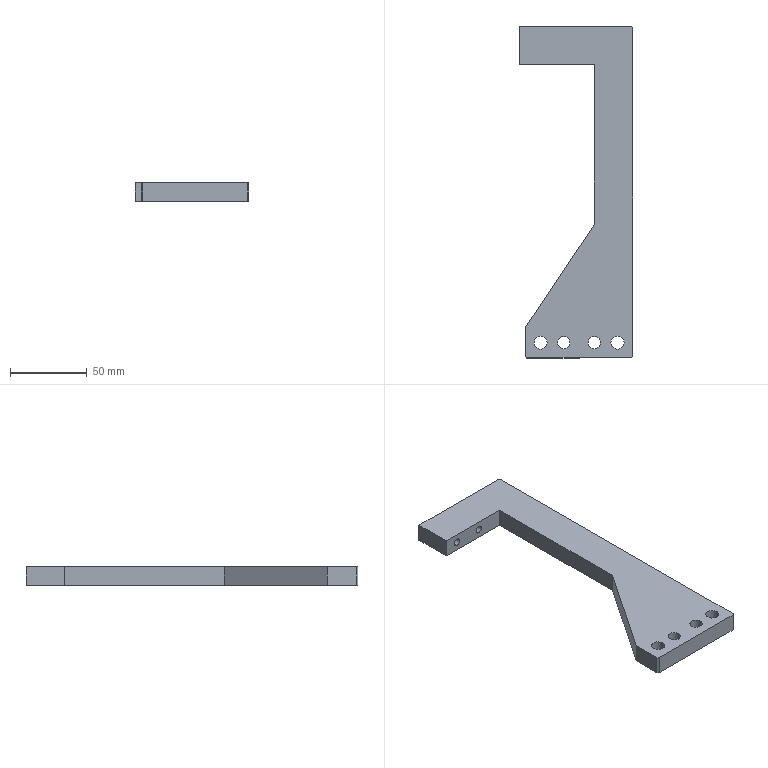Part | SolidWorks | features Chamfer 2, HoleWzd 2, Cut 1, Extrusion 1 | 1 solid | 25 faces | box 74 x 216 x 12 mm | volume 104830 mm3 | plane 13 | cylinder 12 | commonest cylinder face diameters 5 x4 8 x4 8.5 x4
STEP:
#1=CARTESIAN_POINT('',(10.869,171.,-3.5));
#2=VERTEX_POINT('',#1);
#3=CARTESIAN_POINT('',(10.869,171.,-8.5));
#4=VERTEX_POINT('',#3);
#5=CARTESIAN_POINT('',(10.869,171.,-6.));
#6=DIRECTION('',(0.,-1.,0.));
#7=DIRECTION('',(0.,0.,-1.));
#8=AXIS2_PLACEMENT_3D('',#5,#6,#7);
#9=CIRCLE('',#8,2.5);
#10=EDGE_CURVE('',#2,#4,#9,.T.);
#11=ORIENTED_EDGE('',*,*,#10,.T.);
#12=CARTESIAN_POINT('',(10.869,196.,-8.5));
#13=VERTEX_POINT('',#12);
#14=CARTESIAN_POINT('',(10.869,196.,-8.5));
#15=DIRECTION('',(0.,1.,0.));
#16=VECTOR('',#15,1000.);
#17=LINE('',#14,#16);
#18=EDGE_CURVE('',#4,#13,#17,.T.);
#19=ORIENTED_EDGE('',*,*,#18,.T.);
#20=CARTESIAN_POINT('',(10.869,196.,-3.5));
#21=VERTEX_POINT('',#20);
#22=CARTESIAN_POINT('',(10.869,196.,-6.));
#23=DIRECTION('',(0.,1.,0.));
#24=DIRECTION('',(0.,0.,1.));
#25=AXIS2_PLACEMENT_3D('',#22,#23,#24);
#26=CIRCLE('',#25,2.5);
#27=EDGE_CURVE('',#13,#21,#26,.T.);
#28=ORIENTED_EDGE('',*,*,#27,.T.);
#29=CARTESIAN_POINT('',(10.869,196.,-3.5));
#30=DIRECTION('',(0.,1.,0.));
#31=VECTOR('',#30,1000.);
#32=LINE('',#29,#31);
#33=EDGE_CURVE('',#2,#21,#32,.T.);
#34=ORIENTED_EDGE('',*,*,#33,.F.);
#35=EDGE_LOOP('',(#11,#19,#28,#34));
#36=FACE_OUTER_BOUND('',#35,.T.);
#37=CARTESIAN_POINT('',(10.869,196.,-6.));
#38=DIRECTION('',(0.,1.,0.));
#39=DIRECTION('',(0.,0.,1.));
#40=AXIS2_PLACEMENT_3D('',#37,#38,#39);
#41=CYLINDRICAL_SURFACE('',#40,2.5);
#42=ADVANCED_FACE('',(#36),#41,.F.);
#43=CARTESIAN_POINT('',(30.869,171.,-3.5));
#44=VERTEX_POINT('',#43);
#45=CARTESIAN_POINT('',(30.869,171.,-8.5));
#46=VERTEX_POINT('',#45);
#47=CARTESIAN_POINT('',(30.869,171.,-6.));
#48=DIRECTION('',(0.,-1.,0.));
#49=DIRECTION('',(0.,0.,-1.));
#50=AXIS2_PLACEMENT_3D('',#47,#48,#49);
#51=CIRCLE('',#50,2.5);
#52=EDGE_CURVE('',#44,#46,#51,.T.);
#53=ORIENTED_EDGE('',*,*,#52,.T.);
#54=CARTESIAN_POINT('',(30.869,196.,-8.5));
#55=VERTEX_POINT('',#54);
#56=CARTESIAN_POINT('',(30.869,196.,-8.5));
#57=DIRECTION('',(0.,1.,0.));
#58=VECTOR('',#57,1000.);
#59=LINE('',#56,#58);
#60=EDGE_CURVE('',#46,#55,#59,.T.);
#61=ORIENTED_EDGE('',*,*,#60,.T.);
#62=CARTESIAN_POINT('',(30.869,196.,-3.5));
#63=VERTEX_POINT('',#62);
#64=CARTESIAN_POINT('',(30.869,196.,-6.));
#65=DIRECTION('',(0.,1.,0.));
#66=DIRECTION('',(0.,0.,1.));
#67=AXIS2_PLACEMENT_3D('',#64,#65,#66);
#68=CIRCLE('',#67,2.5);
#69=EDGE_CURVE('',#55,#63,#68,.T.);
#70=ORIENTED_EDGE('',*,*,#69,.T.);
#71=CARTESIAN_POINT('',(30.869,196.,-3.5));
#72=DIRECTION('',(0.,1.,0.));
#73=VECTOR('',#72,1000.);
#74=LINE('',#71,#73);
#75=EDGE_CURVE('',#44,#63,#74,.T.);
#76=ORIENTED_EDGE('',*,*,#75,.F.);
#77=EDGE_LOOP('',(#53,#61,#70,#76));
#78=FACE_OUTER_BOUND('',#77,.T.);
#79=CARTESIAN_POINT('',(30.869,196.,-6.));
#80=DIRECTION('',(0.,1.,0.));
#81=DIRECTION('',(0.,0.,1.));
#82=AXIS2_PLACEMENT_3D('',#79,#80,#81);
#83=CYLINDRICAL_SURFACE('',#82,2.5);
#84=ADVANCED_FACE('',(#78),#83,.F.);
#85=CARTESIAN_POINT('',(45.869,-10.,-12.));
#86=VERTEX_POINT('',#85);
#87=CARTESIAN_POINT('',(53.869,-10.,-12.));
#88=VERTEX_POINT('',#87);
#89=CARTESIAN_POINT('',(49.869,-10.,-12.));
#90=DIRECTION('',(0.,0.,1.));
#91=DIRECTION('',(1.,0.,0.));
#92=AXIS2_PLACEMENT_3D('',#89,#90,#91);
#93=CIRCLE('',#92,4.);
#94=EDGE_CURVE('',#86,#88,#93,.T.);
#95=ORIENTED_EDGE('',*,*,#94,.F.);
#96=CARTESIAN_POINT('',(45.869,-10.,0.));
#97=VERTEX_POINT('',#96);
#98=CARTESIAN_POINT('',(45.869,-10.,-12.));
#99=DIRECTION('',(0.,0.,1.));
#100=VECTOR('',#99,1000.);
#101=LINE('',#98,#100);
#102=EDGE_CURVE('',#86,#97,#101,.T.);
#103=ORIENTED_EDGE('',*,*,#102,.T.);
#104=CARTESIAN_POINT('',(53.869,-10.,0.));
#105=VERTEX_POINT('',#104);
#106=CARTESIAN_POINT('',(49.869,-10.,0.));
#107=DIRECTION('',(0.,0.,1.));
#108=DIRECTION('',(1.,0.,0.));
#109=AXIS2_PLACEMENT_3D('',#106,#107,#108);
#110=CIRCLE('',#109,4.);
#111=EDGE_CURVE('',#97,#105,#110,.T.);
#112=ORIENTED_EDGE('',*,*,#111,.T.);
#113=CARTESIAN_POINT('',(53.869,-10.,-12.));
#114=DIRECTION('',(0.,0.,1.));
#115=VECTOR('',#114,1000.);
#116=LINE('',#113,#115);
#117=EDGE_CURVE('',#88,#105,#116,.T.);
#118=ORIENTED_EDGE('',*,*,#117,.F.);
#119=EDGE_LOOP('',(#95,#103,#112,#118));
#120=FACE_OUTER_BOUND('',#119,.T.);
#121=CARTESIAN_POINT('',(49.869,-10.,-12.));
#122=DIRECTION('',(0.,0.,1.));
#123=DIRECTION('',(1.,0.,0.));
#124=AXIS2_PLACEMENT_3D('',#121,#122,#123);
#125=CYLINDRICAL_SURFACE('',#124,4.);
#126=ADVANCED_FACE('',(#120),#125,.F.);
#127=CARTESIAN_POINT('',(25.869,-10.,-12.));
#128=VERTEX_POINT('',#127);
#129=CARTESIAN_POINT('',(33.869,-10.,-12.));
#130=VERTEX_POINT('',#129);
#131=CARTESIAN_POINT('',(29.869,-10.,-12.));
#132=DIRECTION('',(0.,0.,1.));
#133=DIRECTION('',(1.,0.,0.));
#134=AXIS2_PLACEMENT_3D('',#131,#132,#133);
#135=CIRCLE('',#134,4.);
#136=EDGE_CURVE('',#128,#130,#135,.T.);
#137=ORIENTED_EDGE('',*,*,#136,.F.);
#138=CARTESIAN_POINT('',(25.869,-10.,0.));
#139=VERTEX_POINT('',#138);
#140=CARTESIAN_POINT('',(25.869,-10.,-12.));
#141=DIRECTION('',(0.,0.,1.));
#142=VECTOR('',#141,1000.);
#143=LINE('',#140,#142);
#144=EDGE_CURVE('',#128,#139,#143,.T.);
#145=ORIENTED_EDGE('',*,*,#144,.T.);
#146=CARTESIAN_POINT('',(33.869,-10.,0.));
#147=VERTEX_POINT('',#146);
#148=CARTESIAN_POINT('',(29.869,-10.,0.));
#149=DIRECTION('',(0.,0.,1.));
#150=DIRECTION('',(1.,0.,0.));
#151=AXIS2_PLACEMENT_3D('',#148,#149,#150);
#152=CIRCLE('',#151,4.);
#153=EDGE_CURVE('',#139,#147,#152,.T.);
#154=ORIENTED_EDGE('',*,*,#153,.T.);
#155=CARTESIAN_POINT('',(33.869,-10.,-12.));
#156=DIRECTION('',(0.,0.,1.));
#157=VECTOR('',#156,1000.);
#158=LINE('',#155,#157);
#159=EDGE_CURVE('',#130,#147,#158,.T.);
#160=ORIENTED_EDGE('',*,*,#159,.F.);
#161=EDGE_LOOP('',(#137,#145,#154,#160));
#162=FACE_OUTER_BOUND('',#161,.T.);
#163=CARTESIAN_POINT('',(29.869,-10.,-12.));
#164=DIRECTION('',(0.,0.,1.));
#165=DIRECTION('',(1.,0.,0.));
#166=AXIS2_PLACEMENT_3D('',#163,#164,#165);
#167=CYLINDRICAL_SURFACE('',#166,4.);
#168=ADVANCED_FACE('',(#162),#167,.F.);
#169=CARTESIAN_POINT('',(69.119,-10.,-12.));
#170=VERTEX_POINT('',#169);
#171=CARTESIAN_POINT('',(60.619,-10.,-12.));
#172=VERTEX_POINT('',#171);
#173=CARTESIAN_POINT('',(64.869,-10.,-12.));
#174=DIRECTION('',(0.,0.,-1.));
#175=DIRECTION('',(-1.,0.,0.));
#176=AXIS2_PLACEMENT_3D('',#173,#174,#175);
#177=CIRCLE('',#176,4.25);
#178=EDGE_CURVE('',#170,#172,#177,.T.);
#179=ORIENTED_EDGE('',*,*,#178,.T.);
#180=CARTESIAN_POINT('',(60.619,-10.,0.));
#181=VERTEX_POINT('',#180);
#182=CARTESIAN_POINT('',(60.619,-10.,0.));
#183=DIRECTION('',(0.,0.,1.));
#184=VECTOR('',#183,1000.);
#185=LINE('',#182,#184);
#186=EDGE_CURVE('',#172,#181,#185,.T.);
#187=ORIENTED_EDGE('',*,*,#186,.T.);
#188=CARTESIAN_POINT('',(69.119,-10.,0.));
#189=VERTEX_POINT('',#188);
#190=CARTESIAN_POINT('',(64.869,-10.,0.));
#191=DIRECTION('',(0.,0.,1.));
#192=DIRECTION('',(1.,0.,0.));
#193=AXIS2_PLACEMENT_3D('',#190,#191,#192);
#194=CIRCLE('',#193,4.25);
#195=EDGE_CURVE('',#181,#189,#194,.T.);
#196=ORIENTED_EDGE('',*,*,#195,.T.);
#197=CARTESIAN_POINT('',(69.119,-10.,0.));
#198=DIRECTION('',(0.,0.,1.));
#199=VECTOR('',#198,1000.);
#200=LINE('',#197,#199);
#201=EDGE_CURVE('',#170,#189,#200,.T.);
#202=ORIENTED_EDGE('',*,*,#201,.F.);
#203=EDGE_LOOP('',(#179,#187,#196,#202));
#204=FACE_OUTER_BOUND('',#203,.T.);
#205=CARTESIAN_POINT('',(64.869,-10.,0.));
#206=DIRECTION('',(0.,0.,1.));
#207=DIRECTION('',(1.,0.,0.));
#208=AXIS2_PLACEMENT_3D('',#205,#206,#207);
#209=CYLINDRICAL_SURFACE('',#208,4.25);
#210=ADVANCED_FACE('',(#204),#209,.F.);
#211=CARTESIAN_POINT('',(19.119,-10.,-12.));
#212=VERTEX_POINT('',#211);
#213=CARTESIAN_POINT('',(10.619,-10.,-12.));
#214=VERTEX_POINT('',#213);
#215=CARTESIAN_POINT('',(14.869,-10.,-12.));
#216=DIRECTION('',(0.,0.,-1.));
#217=DIRECTION('',(-1.,0.,0.));
#218=AXIS2_PLACEMENT_3D('',#215,#216,#217);
#219=CIRCLE('',#218,4.25);
#220=EDGE_CURVE('',#212,#214,#219,.T.);
#221=ORIENTED_EDGE('',*,*,#220,.T.);
#222=CARTESIAN_POINT('',(10.619,-10.,0.));
#223=VERTEX_POINT('',#222);
#224=CARTESIAN_POINT('',(10.619,-10.,0.));
#225=DIRECTION('',(0.,0.,1.));
#226=VECTOR('',#225,1000.);
#227=LINE('',#224,#226);
#228=EDGE_CURVE('',#214,#223,#227,.T.);
#229=ORIENTED_EDGE('',*,*,#228,.T.);
#230=CARTESIAN_POINT('',(19.119,-10.,0.));
#231=VERTEX_POINT('',#230);
#232=CARTESIAN_POINT('',(14.869,-10.,0.));
#233=DIRECTION('',(0.,0.,1.));
#234=DIRECTION('',(1.,0.,0.));
#235=AXIS2_PLACEMENT_3D('',#232,#233,#234);
#236=CIRCLE('',#235,4.25);
#237=EDGE_CURVE('',#223,#231,#236,.T.);
#238=ORIENTED_EDGE('',*,*,#237,.T.);
#239=CARTESIAN_POINT('',(19.119,-10.,0.));
#240=DIRECTION('',(0.,0.,1.));
#241=VECTOR('',#240,1000.);
#242=LINE('',#239,#241);
#243=EDGE_CURVE('',#212,#231,#242,.T.);
#244=ORIENTED_EDGE('',*,*,#243,.F.);
#245=EDGE_LOOP('',(#221,#229,#238,#244));
#246=FACE_OUTER_BOUND('',#245,.T.);
#247=CARTESIAN_POINT('',(14.869,-10.,0.));
#248=DIRECTION('',(0.,0.,1.));
#249=DIRECTION('',(1.,0.,0.));
#250=AXIS2_PLACEMENT_3D('',#247,#248,#249);
#251=CYLINDRICAL_SURFACE('',#250,4.25);
#252=ADVANCED_FACE('',(#246),#251,.F.);
#253=CARTESIAN_POINT('',(74.869,-19.,0.));
#254=VERTEX_POINT('',#253);
#255=CARTESIAN_POINT('',(74.869,195.,0.));
#256=VERTEX_POINT('',#255);
#257=CARTESIAN_POINT('',(74.869,196.,0.));
#258=DIRECTION('',(0.,1.,0.));
#259=VECTOR('',#258,1000.);
#260=LINE('',#257,#259);
#261=EDGE_CURVE('',#254,#256,#260,.T.);
#262=ORIENTED_EDGE('',*,*,#261,.F.);
#263=CARTESIAN_POINT('',(74.869,-19.,-12.));
#264=VERTEX_POINT('',#263);
#265=CARTESIAN_POINT('',(74.869,-19.,-12.));
#266=DIRECTION('',(0.,0.,-1.));
#267=VECTOR('',#266,1000.);
#268=LINE('',#265,#267);
#269=EDGE_CURVE('',#254,#264,#268,.T.);
#270=ORIENTED_EDGE('',*,*,#269,.T.);
#271=CARTESIAN_POINT('',(74.869,195.,-12.));
#272=VERTEX_POINT('',#271);
#273=CARTESIAN_POINT('',(74.869,196.,-12.));
#274=DIRECTION('',(0.,1.,0.));
#275=VECTOR('',#274,1000.);
#276=LINE('',#273,#275);
#277=EDGE_CURVE('',#264,#272,#276,.T.);
#278=ORIENTED_EDGE('',*,*,#277,.T.);
#279=CARTESIAN_POINT('',(74.869,195.,-12.));
#280=DIRECTION('',(0.,0.,1.));
#281=VECTOR('',#280,1000.);
#282=LINE('',#279,#281);
#283=EDGE_CURVE('',#272,#256,#282,.T.);
#284=ORIENTED_EDGE('',*,*,#283,.T.);
#285=EDGE_LOOP('',(#262,#270,#278,#284));
#286=FACE_OUTER_BOUND('',#285,.T.);
#287=CARTESIAN_POINT('',(74.869,196.,-12.));
#288=DIRECTION('',(1.,0.,0.));
#289=DIRECTION('',(0.,1.,0.));
#290=AXIS2_PLACEMENT_3D('',#287,#288,#289);
#291=PLANE('',#290);
#292=ADVANCED_FACE('',(#286),#291,.T.);
#293=CARTESIAN_POINT('',(5.869,-20.,0.));
#294=VERTEX_POINT('',#293);
#295=CARTESIAN_POINT('',(73.869,-20.,0.));
#296=VERTEX_POINT('',#295);
#297=CARTESIAN_POINT('',(74.869,-20.,0.));
#298=DIRECTION('',(1.,0.,0.));
#299=VECTOR('',#298,1000.);
#300=LINE('',#297,#299);
#301=EDGE_CURVE('',#294,#296,#300,.T.);
#302=ORIENTED_EDGE('',*,*,#301,.F.);
#303=CARTESIAN_POINT('',(5.869,-20.,-12.));
#304=VERTEX_POINT('',#303);
#305=CARTESIAN_POINT('',(5.869,-20.,-12.));
#306=DIRECTION('',(0.,0.,-1.));
#307=VECTOR('',#306,1000.);
#308=LINE('',#305,#307);
#309=EDGE_CURVE('',#294,#304,#308,.T.);
#310=ORIENTED_EDGE('',*,*,#309,.T.);
#311=CARTESIAN_POINT('',(73.869,-20.,-12.));
#312=VERTEX_POINT('',#311);
#313=CARTESIAN_POINT('',(74.869,-20.,-12.));
#314=DIRECTION('',(1.,0.,0.));
#315=VECTOR('',#314,1000.);
#316=LINE('',#313,#315);
#317=EDGE_CURVE('',#304,#312,#316,.T.);
#318=ORIENTED_EDGE('',*,*,#317,.T.);
#319=CARTESIAN_POINT('',(73.869,-20.,-12.));
#320=DIRECTION('',(0.,0.,1.));
#321=VECTOR('',#320,1000.);
#322=LINE('',#319,#321);
#323=EDGE_CURVE('',#312,#296,#322,.T.);
#324=ORIENTED_EDGE('',*,*,#323,.T.);
#325=EDGE_LOOP('',(#302,#310,#318,#324));
#326=FACE_OUTER_BOUND('',#325,.T.);
#327=CARTESIAN_POINT('',(74.869,-20.,-12.));
#328=DIRECTION('',(0.,-1.,0.));
#329=DIRECTION('',(1.,0.,0.));
#330=AXIS2_PLACEMENT_3D('',#327,#328,#329);
#331=PLANE('',#330);
#332=ADVANCED_FACE('',(#326),#331,.T.);
#333=CARTESIAN_POINT('',(4.869,0.,-12.));
#334=VERTEX_POINT('',#333);
#335=CARTESIAN_POINT('',(4.869,-19.,-12.));
#336=VERTEX_POINT('',#335);
#337=CARTESIAN_POINT('',(4.869,-20.,-12.));
#338=DIRECTION('',(0.,-1.,0.));
#339=VECTOR('',#338,1000.);
#340=LINE('',#337,#339);
#341=EDGE_CURVE('',#334,#336,#340,.T.);
#342=ORIENTED_EDGE('',*,*,#341,.T.);
#343=CARTESIAN_POINT('',(4.869,-19.,0.));
#344=VERTEX_POINT('',#343);
#345=CARTESIAN_POINT('',(4.869,-19.,-12.));
#346=DIRECTION('',(0.,0.,1.));
#347=VECTOR('',#346,1000.);
#348=LINE('',#345,#347);
#349=EDGE_CURVE('',#336,#344,#348,.T.);
#350=ORIENTED_EDGE('',*,*,#349,.T.);
#351=CARTESIAN_POINT('',(4.869,0.,0.));
#352=VERTEX_POINT('',#351);
#353=CARTESIAN_POINT('',(4.869,-20.,0.));
#354=DIRECTION('',(0.,-1.,0.));
#355=VECTOR('',#354,1000.);
#356=LINE('',#353,#355);
#357=EDGE_CURVE('',#352,#344,#356,.T.);
#358=ORIENTED_EDGE('',*,*,#357,.F.);
#359=CARTESIAN_POINT('',(4.869,0.,-12.));
#360=DIRECTION('',(0.,0.,1.));
#361=VECTOR('',#360,1000.);
#362=LINE('',#359,#361);
#363=EDGE_CURVE('',#334,#352,#362,.T.);
#364=ORIENTED_EDGE('',*,*,#363,.F.);
#365=EDGE_LOOP('',(#342,#350,#358,#364));
#366=FACE_OUTER_BOUND('',#365,.T.);
#367=CARTESIAN_POINT('',(4.869,-20.,-12.));
#368=DIRECTION('',(-1.,0.,0.));
#369=DIRECTION('',(0.,0.,1.));
#370=AXIS2_PLACEMENT_3D('',#367,#368,#369);
#371=PLANE('',#370);
#372=ADVANCED_FACE('',(#366),#371,.T.);
#373=CARTESIAN_POINT('',(49.869,67.03,0.));
#374=VERTEX_POINT('',#373);
#375=CARTESIAN_POINT('',(4.869,0.,0.));
#376=DIRECTION('',(-0.5574,-0.8303,0.));
#377=VECTOR('',#376,1000.);
#378=LINE('',#375,#377);
#379=EDGE_CURVE('',#374,#352,#378,.T.);
#380=ORIENTED_EDGE('',*,*,#379,.F.);
#381=CARTESIAN_POINT('',(49.869,67.03,-12.));
#382=VERTEX_POINT('',#381);
#383=CARTESIAN_POINT('',(49.869,67.03,-12.));
#384=DIRECTION('',(0.,0.,1.));
#385=VECTOR('',#384,1000.);
#386=LINE('',#383,#385);
#387=EDGE_CURVE('',#382,#374,#386,.T.);
#388=ORIENTED_EDGE('',*,*,#387,.F.);
#389=CARTESIAN_POINT('',(4.869,0.,-12.));
#390=DIRECTION('',(-0.5574,-0.8303,0.));
#391=VECTOR('',#390,1000.);
#392=LINE('',#389,#391);
#393=EDGE_CURVE('',#382,#334,#392,.T.);
#394=ORIENTED_EDGE('',*,*,#393,.T.);
#395=ORIENTED_EDGE('',*,*,#363,.T.);
#396=EDGE_LOOP('',(#380,#388,#394,#395));
#397=FACE_OUTER_BOUND('',#396,.T.);
#398=CARTESIAN_POINT('',(4.869,0.,-12.));
#399=DIRECTION('',(-0.8303,0.5574,0.));
#400=DIRECTION('',(-0.5574,-0.8303,0.));
#401=AXIS2_PLACEMENT_3D('',#398,#399,#400);
#402=PLANE('',#401);
#403=ADVANCED_FACE('',(#397),#402,.T.);
#404=CARTESIAN_POINT('',(49.869,171.,0.));
#405=VERTEX_POINT('',#404);
#406=CARTESIAN_POINT('',(49.869,67.03,0.));
#407=DIRECTION('',(0.,-1.,0.));
#408=VECTOR('',#407,1000.);
#409=LINE('',#406,#408);
#410=EDGE_CURVE('',#405,#374,#409,.T.);
#411=ORIENTED_EDGE('',*,*,#410,.F.);
#412=CARTESIAN_POINT('',(49.869,171.,-12.));
#413=VERTEX_POINT('',#412);
#414=CARTESIAN_POINT('',(49.869,171.,-12.));
#415=DIRECTION('',(0.,0.,1.));
#416=VECTOR('',#415,1000.);
#417=LINE('',#414,#416);
#418=EDGE_CURVE('',#413,#405,#417,.T.);
#419=ORIENTED_EDGE('',*,*,#418,.F.);
#420=CARTESIAN_POINT('',(49.869,67.03,-12.));
#421=DIRECTION('',(0.,-1.,0.));
#422=VECTOR('',#421,1000.);
#423=LINE('',#420,#422);
#424=EDGE_CURVE('',#413,#382,#423,.T.);
#425=ORIENTED_EDGE('',*,*,#424,.T.);
#426=ORIENTED_EDGE('',*,*,#387,.T.);
#427=EDGE_LOOP('',(#411,#419,#425,#426));
#428=FACE_OUTER_BOUND('',#427,.T.);
#429=CARTESIAN_POINT('',(49.869,67.03,-12.));
#430=DIRECTION('',(-1.,0.,0.));
#431=DIRECTION('',(0.,-1.,0.));
#432=AXIS2_PLACEMENT_3D('',#429,#430,#431);
#433=PLANE('',#432);
#434=ADVANCED_FACE('',(#428),#433,.T.);
#435=ORIENTED_EDGE('',*,*,#10,.F.);
#436=CARTESIAN_POINT('',(10.869,171.,-6.));
#437=DIRECTION('',(0.,-1.,0.));
#438=DIRECTION('',(0.,0.,-1.));
#439=AXIS2_PLACEMENT_3D('',#436,#437,#438);
#440=CIRCLE('',#439,2.5);
#441=EDGE_CURVE('',#4,#2,#440,.T.);
#442=ORIENTED_EDGE('',*,*,#441,.F.);
#443=EDGE_LOOP('',(#435,#442));
#444=FACE_BOUND('',#443,.T.);
#445=ORIENTED_EDGE('',*,*,#52,.F.);
#446=CARTESIAN_POINT('',(30.869,171.,-6.));
#447=DIRECTION('',(0.,-1.,0.));
#448=DIRECTION('',(0.,0.,-1.));
#449=AXIS2_PLACEMENT_3D('',#446,#447,#448);
#450=CIRCLE('',#449,2.5);
#451=EDGE_CURVE('',#46,#44,#450,.T.);
#452=ORIENTED_EDGE('',*,*,#451,.F.);
#453=EDGE_LOOP('',(#445,#452));
#454=FACE_BOUND('',#453,.T.);
#455=CARTESIAN_POINT('',(0.8691,171.,0.));
#456=VERTEX_POINT('',#455);
#457=CARTESIAN_POINT('',(49.869,171.,0.));
#458=DIRECTION('',(1.,0.,0.));
#459=VECTOR('',#458,1000.);
#460=LINE('',#457,#459);
#461=EDGE_CURVE('',#456,#405,#460,.T.);
#462=ORIENTED_EDGE('',*,*,#461,.F.);
#463=CARTESIAN_POINT('',(0.8691,171.,-12.));
#464=VERTEX_POINT('',#463);
#465=CARTESIAN_POINT('',(0.8691,171.,-12.));
#466=DIRECTION('',(0.,0.,1.));
#467=VECTOR('',#466,1000.);
#468=LINE('',#465,#467);
#469=EDGE_CURVE('',#464,#456,#468,.T.);
#470=ORIENTED_EDGE('',*,*,#469,.F.);
#471=CARTESIAN_POINT('',(49.869,171.,-12.));
#472=DIRECTION('',(1.,0.,0.));
#473=VECTOR('',#472,1000.);
#474=LINE('',#471,#473);
#475=EDGE_CURVE('',#464,#413,#474,.T.);
#476=ORIENTED_EDGE('',*,*,#475,.T.);
#477=ORIENTED_EDGE('',*,*,#418,.T.);
#478=EDGE_LOOP('',(#462,#470,#476,#477));
#479=FACE_OUTER_BOUND('',#478,.T.);
#480=CARTESIAN_POINT('',(49.869,171.,-12.));
#481=DIRECTION('',(0.,-1.,0.));
#482=DIRECTION('',(0.,0.,-1.));
#483=AXIS2_PLACEMENT_3D('',#480,#481,#482);
#484=PLANE('',#483);
#485=ADVANCED_FACE('',(#444,#454,#479),#484,.T.);
#486=CARTESIAN_POINT('',(0.8691,196.,0.));
#487=VERTEX_POINT('',#486);
#488=CARTESIAN_POINT('',(0.8691,171.,0.));
#489=DIRECTION('',(0.,-1.,0.));
#490=VECTOR('',#489,1000.);
#491=LINE('',#488,#490);
#492=EDGE_CURVE('',#487,#456,#491,.T.);
#493=ORIENTED_EDGE('',*,*,#492,.F.);
#494=CARTESIAN_POINT('',(0.8691,196.,-12.));
#495=VERTEX_POINT('',#494);
#496=CARTESIAN_POINT('',(0.8691,196.,-12.));
#497=DIRECTION('',(0.,0.,1.));
#498=VECTOR('',#497,1000.);
#499=LINE('',#496,#498);
#500=EDGE_CURVE('',#495,#487,#499,.T.);
#501=ORIENTED_EDGE('',*,*,#500,.F.);
#502=CARTESIAN_POINT('',(0.8691,171.,-12.));
#503=DIRECTION('',(0.,-1.,0.));
#504=VECTOR('',#503,1000.);
#505=LINE('',#502,#504);
#506=EDGE_CURVE('',#495,#464,#505,.T.);
#507=ORIENTED_EDGE('',*,*,#506,.T.);
#508=ORIENTED_EDGE('',*,*,#469,.T.);
#509=EDGE_LOOP('',(#493,#501,#507,#508));
#510=FACE_OUTER_BOUND('',#509,.T.);
#511=CARTESIAN_POINT('',(0.8691,171.,-12.));
#512=DIRECTION('',(-1.,0.,0.));
#513=DIRECTION('',(0.,0.,1.));
#514=AXIS2_PLACEMENT_3D('',#511,#512,#513);
#515=PLANE('',#514);
#516=ADVANCED_FACE('',(#510),#515,.T.);
#517=CARTESIAN_POINT('',(10.869,196.,-6.));
#518=DIRECTION('',(0.,1.,0.));
#519=DIRECTION('',(0.,0.,1.));
#520=AXIS2_PLACEMENT_3D('',#517,#518,#519);
#521=CIRCLE('',#520,2.5);
#522=EDGE_CURVE('',#21,#13,#521,.T.);
#523=ORIENTED_EDGE('',*,*,#522,.F.);
#524=ORIENTED_EDGE('',*,*,#27,.F.);
#525=EDGE_LOOP('',(#523,#524));
#526=FACE_BOUND('',#525,.T.);
#527=CARTESIAN_POINT('',(30.869,196.,-6.));
#528=DIRECTION('',(0.,1.,0.));
#529=DIRECTION('',(0.,0.,1.));
#530=AXIS2_PLACEMENT_3D('',#527,#528,#529);
#531=CIRCLE('',#530,2.5);
#532=EDGE_CURVE('',#63,#55,#531,.T.);
#533=ORIENTED_EDGE('',*,*,#532,.F.);
#534=ORIENTED_EDGE('',*,*,#69,.F.);
#535=EDGE_LOOP('',(#533,#534));
#536=FACE_BOUND('',#535,.T.);
#537=CARTESIAN_POINT('',(73.869,196.,0.));
#538=VERTEX_POINT('',#537);
#539=CARTESIAN_POINT('',(0.8691,196.,0.));
#540=DIRECTION('',(-1.,0.,0.));
#541=VECTOR('',#540,1000.);
#542=LINE('',#539,#541);
#543=EDGE_CURVE('',#538,#487,#542,.T.);
#544=ORIENTED_EDGE('',*,*,#543,.F.);
#545=CARTESIAN_POINT('',(73.869,196.,-12.));
#546=VERTEX_POINT('',#545);
#547=CARTESIAN_POINT('',(73.869,196.,-12.));
#548=DIRECTION('',(0.,0.,-1.));
#549=VECTOR('',#548,1000.);
#550=LINE('',#547,#549);
#551=EDGE_CURVE('',#538,#546,#550,.T.);
#552=ORIENTED_EDGE('',*,*,#551,.T.);
#553=CARTESIAN_POINT('',(0.8691,196.,-12.));
#554=DIRECTION('',(-1.,0.,0.));
#555=VECTOR('',#554,1000.);
#556=LINE('',#553,#555);
#557=EDGE_CURVE('',#546,#495,#556,.T.);
#558=ORIENTED_EDGE('',*,*,#557,.T.);
#559=ORIENTED_EDGE('',*,*,#500,.T.);
#560=EDGE_LOOP('',(#544,#552,#558,#559));
#561=FACE_OUTER_BOUND('',#560,.T.);
#562=CARTESIAN_POINT('',(0.8691,196.,-12.));
#563=DIRECTION('',(0.,1.,0.));
#564=DIRECTION('',(0.,0.,1.));
#565=AXIS2_PLACEMENT_3D('',#562,#563,#564);
#566=PLANE('',#565);
#567=ADVANCED_FACE('',(#526,#536,#561),#566,.T.);
#568=CARTESIAN_POINT('',(49.869,-10.,-12.));
#569=DIRECTION('',(0.,0.,1.));
#570=DIRECTION('',(1.,0.,0.));
#571=AXIS2_PLACEMENT_3D('',#568,#569,#570);
#572=CIRCLE('',#571,4.);
#573=EDGE_CURVE('',#88,#86,#572,.T.);
#574=ORIENTED_EDGE('',*,*,#573,.T.);
#575=ORIENTED_EDGE('',*,*,#94,.T.);
#576=EDGE_LOOP('',(#574,#575));
#577=FACE_BOUND('',#576,.T.);
#578=CARTESIAN_POINT('',(29.869,-10.,-12.));
#579=DIRECTION('',(0.,0.,1.));
#580=DIRECTION('',(1.,0.,0.));
#581=AXIS2_PLACEMENT_3D('',#578,#579,#580);
#582=CIRCLE('',#581,4.);
#583=EDGE_CURVE('',#130,#128,#582,.T.);
#584=ORIENTED_EDGE('',*,*,#583,.T.);
#585=ORIENTED_EDGE('',*,*,#136,.T.);
#586=EDGE_LOOP('',(#584,#585));
#587=FACE_BOUND('',#586,.T.);
#588=ORIENTED_EDGE('',*,*,#178,.F.);
#589=CARTESIAN_POINT('',(64.869,-10.,-12.));
#590=DIRECTION('',(0.,0.,-1.));
#591=DIRECTION('',(-1.,0.,0.));
#592=AXIS2_PLACEMENT_3D('',#589,#590,#591);
#593=CIRCLE('',#592,4.25);
#594=EDGE_CURVE('',#172,#170,#593,.T.);
#595=ORIENTED_EDGE('',*,*,#594,.F.);
#596=EDGE_LOOP('',(#588,#595));
#597=FACE_BOUND('',#596,.T.);
#598=ORIENTED_EDGE('',*,*,#220,.F.);
#599=CARTESIAN_POINT('',(14.869,-10.,-12.));
#600=DIRECTION('',(0.,0.,-1.));
#601=DIRECTION('',(-1.,0.,0.));
#602=AXIS2_PLACEMENT_3D('',#599,#600,#601);
#603=CIRCLE('',#602,4.25);
#604=EDGE_CURVE('',#214,#212,#603,.T.);
#605=ORIENTED_EDGE('',*,*,#604,.F.);
#606=EDGE_LOOP('',(#598,#605));
#607=FACE_BOUND('',#606,.T.);
#608=ORIENTED_EDGE('',*,*,#317,.F.);
#609=CARTESIAN_POINT('',(-7.065,-7.065,-12.));
#610=DIRECTION('',(-0.7071,0.7071,0.));
#611=VECTOR('',#610,1000.);
#612=LINE('',#609,#611);
#613=EDGE_CURVE('',#304,#336,#612,.T.);
#614=ORIENTED_EDGE('',*,*,#613,.T.);
#615=ORIENTED_EDGE('',*,*,#341,.F.);
#616=ORIENTED_EDGE('',*,*,#393,.F.);
#617=ORIENTED_EDGE('',*,*,#424,.F.);
#618=ORIENTED_EDGE('',*,*,#475,.F.);
#619=ORIENTED_EDGE('',*,*,#506,.F.);
#620=ORIENTED_EDGE('',*,*,#557,.F.);
#621=CARTESIAN_POINT('',(134.935,134.935,-12.));
#622=DIRECTION('',(0.7071,-0.7071,0.));
#623=VECTOR('',#622,1000.);
#624=LINE('',#621,#623);
#625=EDGE_CURVE('',#546,#272,#624,.T.);
#626=ORIENTED_EDGE('',*,*,#625,.T.);
#627=ORIENTED_EDGE('',*,*,#277,.F.);
#628=CARTESIAN_POINT('',(46.935,-46.935,-12.));
#629=DIRECTION('',(-0.7071,-0.7071,0.));
#630=VECTOR('',#629,1000.);
#631=LINE('',#628,#630);
#632=EDGE_CURVE('',#264,#312,#631,.T.);
#633=ORIENTED_EDGE('',*,*,#632,.T.);
#634=EDGE_LOOP('',(#608,#614,#615,#616,#617,#618,#619,#620,#626,#627,#633));
#635=FACE_OUTER_BOUND('',#634,.T.);
#636=CARTESIAN_POINT('',(0.,0.,-12.));
#637=DIRECTION('',(0.,0.,-1.));
#638=DIRECTION('',(-1.,0.,0.));
#639=AXIS2_PLACEMENT_3D('',#636,#637,#638);
#640=PLANE('',#639);
#641=ADVANCED_FACE('',(#577,#587,#597,#607,#635),#640,.T.);
#642=CARTESIAN_POINT('',(49.869,-10.,0.));
#643=DIRECTION('',(0.,0.,1.));
#644=DIRECTION('',(1.,0.,0.));
#645=AXIS2_PLACEMENT_3D('',#642,#643,#644);
#646=CIRCLE('',#645,4.);
#647=EDGE_CURVE('',#105,#97,#646,.T.);
#648=ORIENTED_EDGE('',*,*,#647,.F.);
#649=ORIENTED_EDGE('',*,*,#111,.F.);
#650=EDGE_LOOP('',(#648,#649));
#651=FACE_BOUND('',#650,.T.);
#652=CARTESIAN_POINT('',(29.869,-10.,0.));
#653=DIRECTION('',(0.,0.,1.));
#654=DIRECTION('',(1.,0.,0.));
#655=AXIS2_PLACEMENT_3D('',#652,#653,#654);
#656=CIRCLE('',#655,4.);
#657=EDGE_CURVE('',#147,#139,#656,.T.);
#658=ORIENTED_EDGE('',*,*,#657,.F.);
#659=ORIENTED_EDGE('',*,*,#153,.F.);
#660=EDGE_LOOP('',(#658,#659));
#661=FACE_BOUND('',#660,.T.);
#662=CARTESIAN_POINT('',(64.869,-10.,0.));
#663=DIRECTION('',(0.,0.,1.));
#664=DIRECTION('',(1.,0.,0.));
#665=AXIS2_PLACEMENT_3D('',#662,#663,#664);
#666=CIRCLE('',#665,4.25);
#667=EDGE_CURVE('',#189,#181,#666,.T.);
#668=ORIENTED_EDGE('',*,*,#667,.F.);
#669=ORIENTED_EDGE('',*,*,#195,.F.);
#670=EDGE_LOOP('',(#668,#669));
#671=FACE_BOUND('',#670,.T.);
#672=CARTESIAN_POINT('',(14.869,-10.,0.));
#673=DIRECTION('',(0.,0.,1.));
#674=DIRECTION('',(1.,0.,0.));
#675=AXIS2_PLACEMENT_3D('',#672,#673,#674);
#676=CIRCLE('',#675,4.25);
#677=EDGE_CURVE('',#231,#223,#676,.T.);
#678=ORIENTED_EDGE('',*,*,#677,.F.);
#679=ORIENTED_EDGE('',*,*,#237,.F.);
#680=EDGE_LOOP('',(#678,#679));
#681=FACE_BOUND('',#680,.T.);
#682=ORIENTED_EDGE('',*,*,#357,.T.);
#683=CARTESIAN_POINT('',(4.869,-19.,0.));
#684=DIRECTION('',(0.7071,-0.7071,0.));
#685=VECTOR('',#684,1000.);
#686=LINE('',#683,#685);
#687=EDGE_CURVE('',#344,#294,#686,.T.);
#688=ORIENTED_EDGE('',*,*,#687,.T.);
#689=ORIENTED_EDGE('',*,*,#301,.T.);
#690=CARTESIAN_POINT('',(73.869,-20.,0.));
#691=DIRECTION('',(0.7071,0.7071,0.));
#692=VECTOR('',#691,1000.);
#693=LINE('',#690,#692);
#694=EDGE_CURVE('',#296,#254,#693,.T.);
#695=ORIENTED_EDGE('',*,*,#694,.T.);
#696=ORIENTED_EDGE('',*,*,#261,.T.);
#697=CARTESIAN_POINT('',(74.869,195.,0.));
#698=DIRECTION('',(-0.7071,0.7071,0.));
#699=VECTOR('',#698,1000.);
#700=LINE('',#697,#699);
#701=EDGE_CURVE('',#256,#538,#700,.T.);
#702=ORIENTED_EDGE('',*,*,#701,.T.);
#703=ORIENTED_EDGE('',*,*,#543,.T.);
#704=ORIENTED_EDGE('',*,*,#492,.T.);
#705=ORIENTED_EDGE('',*,*,#461,.T.);
#706=ORIENTED_EDGE('',*,*,#410,.T.);
#707=ORIENTED_EDGE('',*,*,#379,.T.);
#708=EDGE_LOOP('',(#682,#688,#689,#695,#696,#702,#703,#704,#705,#706,#707));
#709=FACE_OUTER_BOUND('',#708,.T.);
#710=CARTESIAN_POINT('',(0.,0.,0.));
#711=DIRECTION('',(0.,0.,-1.));
#712=DIRECTION('',(-1.,0.,0.));
#713=AXIS2_PLACEMENT_3D('',#710,#711,#712);
#714=PLANE('',#713);
#715=ADVANCED_FACE('',(#651,#661,#671,#681,#709),#714,.F.);
#716=ORIENTED_EDGE('',*,*,#228,.F.);
#717=ORIENTED_EDGE('',*,*,#604,.T.);
#718=ORIENTED_EDGE('',*,*,#243,.T.);
#719=ORIENTED_EDGE('',*,*,#677,.T.);
#720=EDGE_LOOP('',(#716,#717,#718,#719));
#721=FACE_OUTER_BOUND('',#720,.T.);
#722=CARTESIAN_POINT('',(14.869,-10.,0.));
#723=DIRECTION('',(0.,0.,1.));
#724=DIRECTION('',(1.,0.,0.));
#725=AXIS2_PLACEMENT_3D('',#722,#723,#724);
#726=CYLINDRICAL_SURFACE('',#725,4.25);
#727=ADVANCED_FACE('',(#721),#726,.F.);
#728=ORIENTED_EDGE('',*,*,#186,.F.);
#729=ORIENTED_EDGE('',*,*,#594,.T.);
#730=ORIENTED_EDGE('',*,*,#201,.T.);
#731=ORIENTED_EDGE('',*,*,#667,.T.);
#732=EDGE_LOOP('',(#728,#729,#730,#731));
#733=FACE_OUTER_BOUND('',#732,.T.);
#734=CARTESIAN_POINT('',(64.869,-10.,0.));
#735=DIRECTION('',(0.,0.,1.));
#736=DIRECTION('',(1.,0.,0.));
#737=AXIS2_PLACEMENT_3D('',#734,#735,#736);
#738=CYLINDRICAL_SURFACE('',#737,4.25);
#739=ADVANCED_FACE('',(#733),#738,.F.);
#740=ORIENTED_EDGE('',*,*,#144,.F.);
#741=ORIENTED_EDGE('',*,*,#583,.F.);
#742=ORIENTED_EDGE('',*,*,#159,.T.);
#743=ORIENTED_EDGE('',*,*,#657,.T.);
#744=EDGE_LOOP('',(#740,#741,#742,#743));
#745=FACE_OUTER_BOUND('',#744,.T.);
#746=CARTESIAN_POINT('',(29.869,-10.,-12.));
#747=DIRECTION('',(0.,0.,1.));
#748=DIRECTION('',(1.,0.,0.));
#749=AXIS2_PLACEMENT_3D('',#746,#747,#748);
#750=CYLINDRICAL_SURFACE('',#749,4.);
#751=ADVANCED_FACE('',(#745),#750,.F.);
#752=ORIENTED_EDGE('',*,*,#102,.F.);
#753=ORIENTED_EDGE('',*,*,#573,.F.);
#754=ORIENTED_EDGE('',*,*,#117,.T.);
#755=ORIENTED_EDGE('',*,*,#647,.T.);
#756=EDGE_LOOP('',(#752,#753,#754,#755));
#757=FACE_OUTER_BOUND('',#756,.T.);
#758=CARTESIAN_POINT('',(49.869,-10.,-12.));
#759=DIRECTION('',(0.,0.,1.));
#760=DIRECTION('',(1.,0.,0.));
#761=AXIS2_PLACEMENT_3D('',#758,#759,#760);
#762=CYLINDRICAL_SURFACE('',#761,4.);
#763=ADVANCED_FACE('',(#757),#762,.F.);
#764=ORIENTED_EDGE('',*,*,#60,.F.);
#765=ORIENTED_EDGE('',*,*,#451,.T.);
#766=ORIENTED_EDGE('',*,*,#75,.T.);
#767=ORIENTED_EDGE('',*,*,#532,.T.);
#768=EDGE_LOOP('',(#764,#765,#766,#767));
#769=FACE_OUTER_BOUND('',#768,.T.);
#770=CARTESIAN_POINT('',(30.869,196.,-6.));
#771=DIRECTION('',(0.,1.,0.));
#772=DIRECTION('',(0.,0.,1.));
#773=AXIS2_PLACEMENT_3D('',#770,#771,#772);
#774=CYLINDRICAL_SURFACE('',#773,2.5);
#775=ADVANCED_FACE('',(#769),#774,.F.);
#776=ORIENTED_EDGE('',*,*,#18,.F.);
#777=ORIENTED_EDGE('',*,*,#441,.T.);
#778=ORIENTED_EDGE('',*,*,#33,.T.);
#779=ORIENTED_EDGE('',*,*,#522,.T.);
#780=EDGE_LOOP('',(#776,#777,#778,#779));
#781=FACE_OUTER_BOUND('',#780,.T.);
#782=CARTESIAN_POINT('',(10.869,196.,-6.));
#783=DIRECTION('',(0.,1.,0.));
#784=DIRECTION('',(0.,0.,1.));
#785=AXIS2_PLACEMENT_3D('',#782,#783,#784);
#786=CYLINDRICAL_SURFACE('',#785,2.5);
#787=ADVANCED_FACE('',(#781),#786,.F.);
#788=ORIENTED_EDGE('',*,*,#632,.F.);
#789=ORIENTED_EDGE('',*,*,#269,.F.);
#790=ORIENTED_EDGE('',*,*,#694,.F.);
#791=ORIENTED_EDGE('',*,*,#323,.F.);
#792=EDGE_LOOP('',(#788,#789,#790,#791));
#793=FACE_OUTER_BOUND('',#792,.T.);
#794=CARTESIAN_POINT('',(73.869,-20.,-12.));
#795=DIRECTION('',(-0.7071,0.7071,0.));
#796=DIRECTION('',(0.,0.,1.));
#797=AXIS2_PLACEMENT_3D('',#794,#795,#796);
#798=PLANE('',#797);
#799=ADVANCED_FACE('',(#793),#798,.F.);
#800=ORIENTED_EDGE('',*,*,#625,.F.);
#801=ORIENTED_EDGE('',*,*,#551,.F.);
#802=ORIENTED_EDGE('',*,*,#701,.F.);
#803=ORIENTED_EDGE('',*,*,#283,.F.);
#804=EDGE_LOOP('',(#800,#801,#802,#803));
#805=FACE_OUTER_BOUND('',#804,.T.);
#806=CARTESIAN_POINT('',(74.869,195.,-12.));
#807=DIRECTION('',(-0.7071,-0.7071,0.));
#808=DIRECTION('',(0.,0.,1.));
#809=AXIS2_PLACEMENT_3D('',#806,#807,#808);
#810=PLANE('',#809);
#811=ADVANCED_FACE('',(#805),#810,.F.);
#812=ORIENTED_EDGE('',*,*,#613,.F.);
#813=ORIENTED_EDGE('',*,*,#309,.F.);
#814=ORIENTED_EDGE('',*,*,#687,.F.);
#815=ORIENTED_EDGE('',*,*,#349,.F.);
#816=EDGE_LOOP('',(#812,#813,#814,#815));
#817=FACE_OUTER_BOUND('',#816,.T.);
#818=CARTESIAN_POINT('',(4.869,-19.,-12.));
#819=DIRECTION('',(0.7071,0.7071,0.));
#820=DIRECTION('',(0.,0.,1.));
#821=AXIS2_PLACEMENT_3D('',#818,#819,#820);
#822=PLANE('',#821);
#823=ADVANCED_FACE('',(#817),#822,.F.);
#824=CLOSED_SHELL('',(#42,#84,#126,#168,#210,#252,#292,#332,#372,#403,#434,#485,#516,#567,#641,#715,#727,#739,#751,#763,#775,#787,#799,#811,#823));
#825=MANIFOLD_SOLID_BREP('',#824);
#826=CARTESIAN_POINT('',(0.,0.,0.));
#827=DIRECTION('',(0.,0.,1.));
#828=DIRECTION('',(1.,0.,0.));
#829=AXIS2_PLACEMENT_3D('',#826,#827,#828);
#830=(LENGTH_UNIT()NAMED_UNIT(*)SI_UNIT(.MILLI.,.METRE.));
#831=UNCERTAINTY_MEASURE_WITH_UNIT(LENGTH_MEASURE(0.00001),#830,'','');
#832=(NAMED_UNIT(*)PLANE_ANGLE_UNIT()SI_UNIT($,.RADIAN.));
#833=(NAMED_UNIT(*)SI_UNIT($,.STERADIAN.)SOLID_ANGLE_UNIT());
#834=(GEOMETRIC_REPRESENTATION_CONTEXT(3)GLOBAL_UNCERTAINTY_ASSIGNED_CONTEXT((#831))GLOBAL_UNIT_ASSIGNED_CONTEXT((#830,#832,#833))REPRESENTATION_CONTEXT('',''));
#835=ADVANCED_BREP_SHAPE_REPRESENTATION('',(#825,#829),#834);